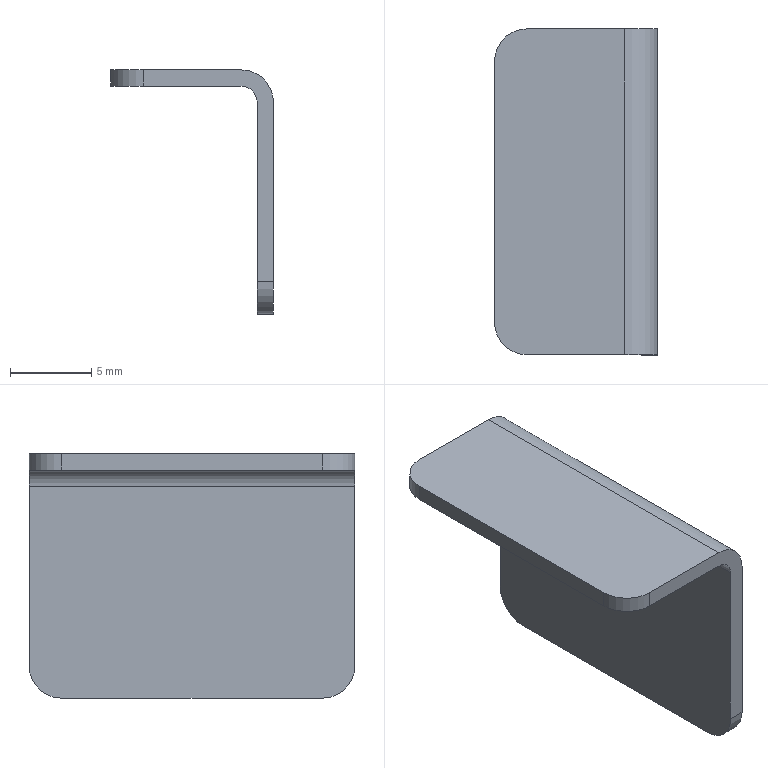Part | STEP file | Tube feed_id198_x_t | 1 solid | 14 faces | box 10 x 20 x 15 mm | volume 463.69 mm3 | plane 8 | cylinder 6 | commonest cylinder face diameters 4 x5 2 x1
STEP:
#1=CARTESIAN_POINT('',(0.,0.,0.));
#2=DIRECTION('',(0.,0.,1.));
#3=DIRECTION('',(1.,0.,0.));
#4=AXIS2_PLACEMENT_3D('',#1,#2,#3);
#5=CARTESIAN_POINT('',(16.,419.936,-21.));
#6=VERTEX_POINT('',#5);
#7=CARTESIAN_POINT('',(16.,403.936,-21.));
#8=VERTEX_POINT('',#7);
#9=CARTESIAN_POINT('',(16.,415.936,-21.));
#10=DIRECTION('',(0.,-1.,0.));
#11=VECTOR('',#10,1.);
#12=LINE('',#9,#11);
#13=CARTESIAN_POINT('',(16.,415.936,-21.));
#14=DIRECTION('',(-1.,0.,0.));
#15=DIRECTION('',(0.,-1.,0.));
#16=AXIS2_PLACEMENT_3D('',#13,#14,#15);
#17=PLANE('',#16);
#18=CARTESIAN_POINT('',(0.,0.));
#19=DIRECTION('',(1.,0.));
#20=VECTOR('',#19,1.);
#21=LINE('',#18,#20);
#22=(GEOMETRIC_REPRESENTATION_CONTEXT(2)PARAMETRIC_REPRESENTATION_CONTEXT()REPRESENTATION_CONTEXT('',''));
#23=DEFINITIONAL_REPRESENTATION('',(#21),#22);
#24=PCURVE('',#17,#23);
#25=CARTESIAN_POINT('',(24.,415.936,-21.));
#26=DIRECTION('',(0.,0.,1.));
#27=DIRECTION('',(1.,0.,0.));
#28=AXIS2_PLACEMENT_3D('',#25,#26,#27);
#29=PLANE('',#28);
#30=CARTESIAN_POINT('',(-8.,0.));
#31=DIRECTION('',(0.,-1.));
#32=VECTOR('',#31,1.);
#33=LINE('',#30,#32);
#34=(GEOMETRIC_REPRESENTATION_CONTEXT(2)PARAMETRIC_REPRESENTATION_CONTEXT()REPRESENTATION_CONTEXT('',''));
#35=DEFINITIONAL_REPRESENTATION('',(#33),#34);
#36=PCURVE('',#29,#35);
#37=SURFACE_CURVE('',#12,(#24,#36),.PCURVE_S1.);
#38=EDGE_CURVE('',#6,#8,#37,.T.);
#39=ORIENTED_EDGE('',*,*,#38,.F.);
#40=CARTESIAN_POINT('',(16.,419.936,-22.));
#41=VERTEX_POINT('',#40);
#42=CARTESIAN_POINT('',(16.,419.936,-21.));
#43=DIRECTION('',(0.,0.,-1.));
#44=VECTOR('',#43,1.);
#45=LINE('',#42,#44);
#46=CARTESIAN_POINT('',(-4.,0.));
#47=DIRECTION('',(0.,-1.));
#48=VECTOR('',#47,1.);
#49=LINE('',#46,#48);
#50=(GEOMETRIC_REPRESENTATION_CONTEXT(2)PARAMETRIC_REPRESENTATION_CONTEXT()REPRESENTATION_CONTEXT('',''));
#51=DEFINITIONAL_REPRESENTATION('',(#49),#50);
#52=PCURVE('',#17,#51);
#53=CARTESIAN_POINT('',(18.,419.936,-21.));
#54=DIRECTION('',(0.,0.,-1.));
#55=DIRECTION('',(-1.,0.,0.));
#56=AXIS2_PLACEMENT_3D('',#53,#54,#55);
#57=CYLINDRICAL_SURFACE('',#56,2.);
#58=CARTESIAN_POINT('',(0.,0.));
#59=DIRECTION('',(0.,1.));
#60=VECTOR('',#59,1.);
#61=LINE('',#58,#60);
#62=(GEOMETRIC_REPRESENTATION_CONTEXT(2)PARAMETRIC_REPRESENTATION_CONTEXT()REPRESENTATION_CONTEXT('',''));
#63=DEFINITIONAL_REPRESENTATION('',(#61),#62);
#64=PCURVE('',#57,#63);
#65=SURFACE_CURVE('',#45,(#52,#64),.PCURVE_S1.);
#66=EDGE_CURVE('',#6,#41,#65,.T.);
#67=ORIENTED_EDGE('',*,*,#66,.T.);
#68=CARTESIAN_POINT('',(16.,403.936,-22.));
#69=VERTEX_POINT('',#68);
#70=CARTESIAN_POINT('',(16.,415.936,-22.));
#71=DIRECTION('',(0.,-1.,0.));
#72=VECTOR('',#71,1.);
#73=LINE('',#70,#72);
#74=CARTESIAN_POINT('',(0.,-1.));
#75=DIRECTION('',(1.,0.));
#76=VECTOR('',#75,1.);
#77=LINE('',#74,#76);
#78=(GEOMETRIC_REPRESENTATION_CONTEXT(2)PARAMETRIC_REPRESENTATION_CONTEXT()REPRESENTATION_CONTEXT('',''));
#79=DEFINITIONAL_REPRESENTATION('',(#77),#78);
#80=PCURVE('',#17,#79);
#81=CARTESIAN_POINT('',(24.,415.936,-22.));
#82=DIRECTION('',(0.,0.,1.));
#83=DIRECTION('',(1.,0.,0.));
#84=AXIS2_PLACEMENT_3D('',#81,#82,#83);
#85=PLANE('',#84);
#86=CARTESIAN_POINT('',(-8.,0.));
#87=DIRECTION('',(0.,-1.));
#88=VECTOR('',#87,1.);
#89=LINE('',#86,#88);
#90=(GEOMETRIC_REPRESENTATION_CONTEXT(2)PARAMETRIC_REPRESENTATION_CONTEXT()REPRESENTATION_CONTEXT('',''));
#91=DEFINITIONAL_REPRESENTATION('',(#89),#90);
#92=PCURVE('',#85,#91);
#93=SURFACE_CURVE('',#73,(#80,#92),.PCURVE_S1.);
#94=EDGE_CURVE('',#41,#69,#93,.T.);
#95=ORIENTED_EDGE('',*,*,#94,.T.);
#96=CARTESIAN_POINT('',(16.,403.936,-21.));
#97=DIRECTION('',(0.,0.,1.));
#98=VECTOR('',#97,1.);
#99=LINE('',#96,#98);
#100=CARTESIAN_POINT('',(12.,0.));
#101=DIRECTION('',(0.,1.));
#102=VECTOR('',#101,1.);
#103=LINE('',#100,#102);
#104=(GEOMETRIC_REPRESENTATION_CONTEXT(2)PARAMETRIC_REPRESENTATION_CONTEXT()REPRESENTATION_CONTEXT('',''));
#105=DEFINITIONAL_REPRESENTATION('',(#103),#104);
#106=PCURVE('',#17,#105);
#107=CARTESIAN_POINT('',(18.,403.936,-23.));
#108=DIRECTION('',(0.,0.,1.));
#109=DIRECTION('',(0.,-1.,0.));
#110=AXIS2_PLACEMENT_3D('',#107,#108,#109);
#111=CYLINDRICAL_SURFACE('',#110,2.);
#112=CARTESIAN_POINT('',(4.712,2.));
#113=DIRECTION('',(0.,1.));
#114=VECTOR('',#113,1.);
#115=LINE('',#112,#114);
#116=(GEOMETRIC_REPRESENTATION_CONTEXT(2)PARAMETRIC_REPRESENTATION_CONTEXT()REPRESENTATION_CONTEXT('',''));
#117=DEFINITIONAL_REPRESENTATION('',(#115),#116);
#118=PCURVE('',#111,#117);
#119=SURFACE_CURVE('',#99,(#106,#118),.PCURVE_S1.);
#120=EDGE_CURVE('',#69,#8,#119,.T.);
#121=ORIENTED_EDGE('',*,*,#120,.T.);
#122=EDGE_LOOP('',(#39,#67,#95,#121));
#123=FACE_BOUND('',#122,.T.);
#124=ADVANCED_FACE('',(#123),#17,.T.);
#125=CARTESIAN_POINT('',(24.,421.936,-22.));
#126=VERTEX_POINT('',#125);
#127=CARTESIAN_POINT('',(18.,421.936,-22.));
#128=VERTEX_POINT('',#127);
#129=CARTESIAN_POINT('',(24.,421.936,-22.));
#130=DIRECTION('',(-1.,0.,0.));
#131=VECTOR('',#130,1.);
#132=LINE('',#129,#131);
#133=CARTESIAN_POINT('',(0.,421.936,0.));
#134=DIRECTION('',(0.,1.,0.));
#135=DIRECTION('',(0.,0.,1.));
#136=AXIS2_PLACEMENT_3D('',#133,#134,#135);
#137=PLANE('',#136);
#138=CARTESIAN_POINT('',(-22.,24.));
#139=DIRECTION('',(0.,-1.));
#140=VECTOR('',#139,1.);
#141=LINE('',#138,#140);
#142=(GEOMETRIC_REPRESENTATION_CONTEXT(2)PARAMETRIC_REPRESENTATION_CONTEXT()REPRESENTATION_CONTEXT('',''));
#143=DEFINITIONAL_REPRESENTATION('',(#141),#142);
#144=PCURVE('',#137,#143);
#145=CARTESIAN_POINT('',(0.,6.));
#146=DIRECTION('',(-1.,0.));
#147=VECTOR('',#146,1.);
#148=LINE('',#145,#147);
#149=(GEOMETRIC_REPRESENTATION_CONTEXT(2)PARAMETRIC_REPRESENTATION_CONTEXT()REPRESENTATION_CONTEXT('',''));
#150=DEFINITIONAL_REPRESENTATION('',(#148),#149);
#151=PCURVE('',#85,#150);
#152=SURFACE_CURVE('',#132,(#144,#151),.PCURVE_S1.);
#153=EDGE_CURVE('',#126,#128,#152,.T.);
#154=ORIENTED_EDGE('',*,*,#153,.T.);
#155=CARTESIAN_POINT('',(18.,421.936,-21.));
#156=VERTEX_POINT('',#155);
#157=CARTESIAN_POINT('',(18.,421.936,0.));
#158=DIRECTION('',(0.,0.,1.));
#159=VECTOR('',#158,1.);
#160=LINE('',#157,#159);
#161=CARTESIAN_POINT('',(0.,18.));
#162=DIRECTION('',(1.,0.));
#163=VECTOR('',#162,1.);
#164=LINE('',#161,#163);
#165=(GEOMETRIC_REPRESENTATION_CONTEXT(2)PARAMETRIC_REPRESENTATION_CONTEXT()REPRESENTATION_CONTEXT('',''));
#166=DEFINITIONAL_REPRESENTATION('',(#164),#165);
#167=PCURVE('',#137,#166);
#168=CARTESIAN_POINT('',(1.571,-21.));
#169=DIRECTION('',(0.,-1.));
#170=VECTOR('',#169,1.);
#171=LINE('',#168,#170);
#172=(GEOMETRIC_REPRESENTATION_CONTEXT(2)PARAMETRIC_REPRESENTATION_CONTEXT()REPRESENTATION_CONTEXT('',''));
#173=DEFINITIONAL_REPRESENTATION('',(#171),#172);
#174=PCURVE('',#57,#173);
#175=SURFACE_CURVE('',#160,(#167,#174),.PCURVE_S1.);
#176=EDGE_CURVE('',#128,#156,#175,.T.);
#177=ORIENTED_EDGE('',*,*,#176,.T.);
#178=CARTESIAN_POINT('',(24.,421.936,-21.));
#179=VERTEX_POINT('',#178);
#180=CARTESIAN_POINT('',(24.,421.936,-21.));
#181=DIRECTION('',(-1.,0.,0.));
#182=VECTOR('',#181,1.);
#183=LINE('',#180,#182);
#184=CARTESIAN_POINT('',(-21.,24.));
#185=DIRECTION('',(0.,-1.));
#186=VECTOR('',#185,1.);
#187=LINE('',#184,#186);
#188=(GEOMETRIC_REPRESENTATION_CONTEXT(2)PARAMETRIC_REPRESENTATION_CONTEXT()REPRESENTATION_CONTEXT('',''));
#189=DEFINITIONAL_REPRESENTATION('',(#187),#188);
#190=PCURVE('',#137,#189);
#191=CARTESIAN_POINT('',(0.,6.));
#192=DIRECTION('',(-1.,0.));
#193=VECTOR('',#192,1.);
#194=LINE('',#191,#193);
#195=(GEOMETRIC_REPRESENTATION_CONTEXT(2)PARAMETRIC_REPRESENTATION_CONTEXT()REPRESENTATION_CONTEXT('',''));
#196=DEFINITIONAL_REPRESENTATION('',(#194),#195);
#197=PCURVE('',#29,#196);
#198=SURFACE_CURVE('',#183,(#190,#197),.PCURVE_S1.);
#199=EDGE_CURVE('',#179,#156,#198,.T.);
#200=ORIENTED_EDGE('',*,*,#199,.F.);
#201=CARTESIAN_POINT('',(26.,421.936,-23.));
#202=VERTEX_POINT('',#201);
#203=CARTESIAN_POINT('',(24.,421.936,-23.));
#204=DIRECTION('',(0.,-1.,0.));
#205=DIRECTION('',(0.,0.,1.));
#206=AXIS2_PLACEMENT_3D('',#203,#204,#205);
#207=CIRCLE('',#206,2.);
#208=CARTESIAN_POINT('',(-21.,24.));
#209=CARTESIAN_POINT('',(-21.,20.536));
#210=CARTESIAN_POINT('',(-24.,22.268));
#211=CARTESIAN_POINT('',(-27.,24.));
#212=CARTESIAN_POINT('',(-24.,25.732));
#213=CARTESIAN_POINT('',(-21.,27.464));
#214=CARTESIAN_POINT('',(-21.,24.));
#215=(BOUNDED_CURVE()B_SPLINE_CURVE(2,(#208,#209,#210,#211,#212,#213,#214),.UNSPECIFIED.,.T.,.F.)B_SPLINE_CURVE_WITH_KNOTS((1,2,2,2,2,1),(-2.094,0.,2.094,4.189,6.283,8.378),.UNSPECIFIED.)CURVE()GEOMETRIC_REPRESENTATION_ITEM()RATIONAL_B_SPLINE_CURVE((1.,0.5,1.,0.5,1.,0.5,1.))REPRESENTATION_ITEM(''));
#216=(GEOMETRIC_REPRESENTATION_CONTEXT(2)PARAMETRIC_REPRESENTATION_CONTEXT()REPRESENTATION_CONTEXT('',''));
#217=DEFINITIONAL_REPRESENTATION('',(#215),#216);
#218=PCURVE('',#137,#217);
#219=CARTESIAN_POINT('',(24.,415.936,-23.));
#220=DIRECTION('',(0.,-1.,0.));
#221=DIRECTION('',(0.,0.,-1.));
#222=AXIS2_PLACEMENT_3D('',#219,#220,#221);
#223=CYLINDRICAL_SURFACE('',#222,2.);
#224=CARTESIAN_POINT('',(-3.142,-6.));
#225=DIRECTION('',(1.,0.));
#226=VECTOR('',#225,1.);
#227=LINE('',#224,#226);
#228=(GEOMETRIC_REPRESENTATION_CONTEXT(2)PARAMETRIC_REPRESENTATION_CONTEXT()REPRESENTATION_CONTEXT('',''));
#229=DEFINITIONAL_REPRESENTATION('',(#227),#228);
#230=PCURVE('',#223,#229);
#231=SURFACE_CURVE('',#207,(#218,#230),.PCURVE_S1.);
#232=EDGE_CURVE('',#202,#179,#231,.T.);
#233=ORIENTED_EDGE('',*,*,#232,.F.);
#234=CARTESIAN_POINT('',(26.,421.936,-34.));
#235=VERTEX_POINT('',#234);
#236=CARTESIAN_POINT('',(26.,421.936,-36.));
#237=DIRECTION('',(0.,0.,1.));
#238=VECTOR('',#237,1.);
#239=LINE('',#236,#238);
#240=CARTESIAN_POINT('',(-36.,26.));
#241=DIRECTION('',(1.,0.));
#242=VECTOR('',#241,1.);
#243=LINE('',#240,#242);
#244=(GEOMETRIC_REPRESENTATION_CONTEXT(2)PARAMETRIC_REPRESENTATION_CONTEXT()REPRESENTATION_CONTEXT('',''));
#245=DEFINITIONAL_REPRESENTATION('',(#243),#244);
#246=PCURVE('',#137,#245);
#247=CARTESIAN_POINT('',(26.,415.936,-36.));
#248=DIRECTION('',(1.,0.,0.));
#249=DIRECTION('',(0.,0.,-1.));
#250=AXIS2_PLACEMENT_3D('',#247,#248,#249);
#251=PLANE('',#250);
#252=CARTESIAN_POINT('',(0.,6.));
#253=DIRECTION('',(-1.,0.));
#254=VECTOR('',#253,1.);
#255=LINE('',#252,#254);
#256=(GEOMETRIC_REPRESENTATION_CONTEXT(2)PARAMETRIC_REPRESENTATION_CONTEXT()REPRESENTATION_CONTEXT('',''));
#257=DEFINITIONAL_REPRESENTATION('',(#255),#256);
#258=PCURVE('',#251,#257);
#259=SURFACE_CURVE('',#239,(#246,#258),.PCURVE_S1.);
#260=EDGE_CURVE('',#235,#202,#259,.T.);
#261=ORIENTED_EDGE('',*,*,#260,.F.);
#262=CARTESIAN_POINT('',(25.,421.936,-34.));
#263=VERTEX_POINT('',#262);
#264=CARTESIAN_POINT('',(0.,421.936,-34.));
#265=DIRECTION('',(-1.,0.,0.));
#266=VECTOR('',#265,1.);
#267=LINE('',#264,#266);
#268=CARTESIAN_POINT('',(-34.,0.));
#269=DIRECTION('',(0.,-1.));
#270=VECTOR('',#269,1.);
#271=LINE('',#268,#270);
#272=(GEOMETRIC_REPRESENTATION_CONTEXT(2)PARAMETRIC_REPRESENTATION_CONTEXT()REPRESENTATION_CONTEXT('',''));
#273=DEFINITIONAL_REPRESENTATION('',(#271),#272);
#274=PCURVE('',#137,#273);
#275=CARTESIAN_POINT('',(0.,419.936,-34.));
#276=DIRECTION('',(1.,0.,0.));
#277=DIRECTION('',(0.,0.,-1.));
#278=AXIS2_PLACEMENT_3D('',#275,#276,#277);
#279=CYLINDRICAL_SURFACE('',#278,2.);
#280=CARTESIAN_POINT('',(1.571,0.));
#281=DIRECTION('',(0.,-1.));
#282=VECTOR('',#281,1.);
#283=LINE('',#280,#282);
#284=(GEOMETRIC_REPRESENTATION_CONTEXT(2)PARAMETRIC_REPRESENTATION_CONTEXT()REPRESENTATION_CONTEXT('',''));
#285=DEFINITIONAL_REPRESENTATION('',(#283),#284);
#286=PCURVE('',#279,#285);
#287=SURFACE_CURVE('',#267,(#274,#286),.PCURVE_S1.);
#288=EDGE_CURVE('',#235,#263,#287,.T.);
#289=ORIENTED_EDGE('',*,*,#288,.T.);
#290=CARTESIAN_POINT('',(25.,421.936,-23.));
#291=VERTEX_POINT('',#290);
#292=CARTESIAN_POINT('',(25.,421.936,-36.));
#293=DIRECTION('',(0.,0.,1.));
#294=VECTOR('',#293,1.);
#295=LINE('',#292,#294);
#296=CARTESIAN_POINT('',(-36.,25.));
#297=DIRECTION('',(1.,0.));
#298=VECTOR('',#297,1.);
#299=LINE('',#296,#298);
#300=(GEOMETRIC_REPRESENTATION_CONTEXT(2)PARAMETRIC_REPRESENTATION_CONTEXT()REPRESENTATION_CONTEXT('',''));
#301=DEFINITIONAL_REPRESENTATION('',(#299),#300);
#302=PCURVE('',#137,#301);
#303=CARTESIAN_POINT('',(25.,415.936,-36.));
#304=DIRECTION('',(1.,0.,0.));
#305=DIRECTION('',(0.,0.,-1.));
#306=AXIS2_PLACEMENT_3D('',#303,#304,#305);
#307=PLANE('',#306);
#308=CARTESIAN_POINT('',(0.,6.));
#309=DIRECTION('',(-1.,0.));
#310=VECTOR('',#309,1.);
#311=LINE('',#308,#310);
#312=(GEOMETRIC_REPRESENTATION_CONTEXT(2)PARAMETRIC_REPRESENTATION_CONTEXT()REPRESENTATION_CONTEXT('',''));
#313=DEFINITIONAL_REPRESENTATION('',(#311),#312);
#314=PCURVE('',#307,#313);
#315=SURFACE_CURVE('',#295,(#302,#314),.PCURVE_S1.);
#316=EDGE_CURVE('',#263,#291,#315,.T.);
#317=ORIENTED_EDGE('',*,*,#316,.T.);
#318=CARTESIAN_POINT('',(24.,421.936,-23.));
#319=DIRECTION('',(0.,-1.,0.));
#320=DIRECTION('',(0.,0.,1.));
#321=AXIS2_PLACEMENT_3D('',#318,#319,#320);
#322=CIRCLE('',#321,1.);
#323=CARTESIAN_POINT('',(-22.,24.));
#324=CARTESIAN_POINT('',(-22.,22.268));
#325=CARTESIAN_POINT('',(-23.5,23.134));
#326=CARTESIAN_POINT('',(-25.,24.));
#327=CARTESIAN_POINT('',(-23.5,24.866));
#328=CARTESIAN_POINT('',(-22.,25.732));
#329=CARTESIAN_POINT('',(-22.,24.));
#330=(BOUNDED_CURVE()B_SPLINE_CURVE(2,(#323,#324,#325,#326,#327,#328,#329),.UNSPECIFIED.,.T.,.F.)B_SPLINE_CURVE_WITH_KNOTS((1,2,2,2,2,1),(-2.094,0.,2.094,4.189,6.283,8.378),.UNSPECIFIED.)CURVE()GEOMETRIC_REPRESENTATION_ITEM()RATIONAL_B_SPLINE_CURVE((1.,0.5,1.,0.5,1.,0.5,1.))REPRESENTATION_ITEM(''));
#331=(GEOMETRIC_REPRESENTATION_CONTEXT(2)PARAMETRIC_REPRESENTATION_CONTEXT()REPRESENTATION_CONTEXT('',''));
#332=DEFINITIONAL_REPRESENTATION('',(#330),#331);
#333=PCURVE('',#137,#332);
#334=CARTESIAN_POINT('',(24.,415.936,-23.));
#335=DIRECTION('',(0.,-1.,0.));
#336=DIRECTION('',(0.,0.,-1.));
#337=AXIS2_PLACEMENT_3D('',#334,#335,#336);
#338=CYLINDRICAL_SURFACE('',#337,1.);
#339=CARTESIAN_POINT('',(-3.142,-6.));
#340=DIRECTION('',(1.,0.));
#341=VECTOR('',#340,1.);
#342=LINE('',#339,#341);
#343=(GEOMETRIC_REPRESENTATION_CONTEXT(2)PARAMETRIC_REPRESENTATION_CONTEXT()REPRESENTATION_CONTEXT('',''));
#344=DEFINITIONAL_REPRESENTATION('',(#342),#343);
#345=PCURVE('',#338,#344);
#346=SURFACE_CURVE('',#322,(#333,#345),.PCURVE_S1.);
#347=EDGE_CURVE('',#291,#126,#346,.T.);
#348=ORIENTED_EDGE('',*,*,#347,.T.);
#349=EDGE_LOOP('',(#154,#177,#200,#233,#261,#289,#317,#348));
#350=FACE_BOUND('',#349,.T.);
#351=ADVANCED_FACE('',(#350),#137,.T.);
#352=CARTESIAN_POINT('',(26.,419.936,-36.));
#353=VERTEX_POINT('',#352);
#354=CARTESIAN_POINT('',(26.,403.936,-36.));
#355=VERTEX_POINT('',#354);
#356=CARTESIAN_POINT('',(26.,415.936,-36.));
#357=DIRECTION('',(0.,-1.,0.));
#358=VECTOR('',#357,1.);
#359=LINE('',#356,#358);
#360=CARTESIAN_POINT('',(26.,415.936,-36.));
#361=DIRECTION('',(0.,0.,1.));
#362=DIRECTION('',(0.,-1.,0.));
#363=AXIS2_PLACEMENT_3D('',#360,#361,#362);
#364=PLANE('',#363);
#365=CARTESIAN_POINT('',(0.,0.));
#366=DIRECTION('',(1.,0.));
#367=VECTOR('',#366,1.);
#368=LINE('',#365,#367);
#369=(GEOMETRIC_REPRESENTATION_CONTEXT(2)PARAMETRIC_REPRESENTATION_CONTEXT()REPRESENTATION_CONTEXT('',''));
#370=DEFINITIONAL_REPRESENTATION('',(#368),#369);
#371=PCURVE('',#364,#370);
#372=CARTESIAN_POINT('',(0.,0.));
#373=DIRECTION('',(0.,-1.));
#374=VECTOR('',#373,1.);
#375=LINE('',#372,#374);
#376=(GEOMETRIC_REPRESENTATION_CONTEXT(2)PARAMETRIC_REPRESENTATION_CONTEXT()REPRESENTATION_CONTEXT('',''));
#377=DEFINITIONAL_REPRESENTATION('',(#375),#376);
#378=PCURVE('',#251,#377);
#379=SURFACE_CURVE('',#359,(#371,#378),.PCURVE_S1.);
#380=EDGE_CURVE('',#353,#355,#379,.T.);
#381=ORIENTED_EDGE('',*,*,#380,.T.);
#382=CARTESIAN_POINT('',(25.,403.936,-36.));
#383=VERTEX_POINT('',#382);
#384=CARTESIAN_POINT('',(26.,403.936,-36.));
#385=DIRECTION('',(-1.,0.,0.));
#386=VECTOR('',#385,1.);
#387=LINE('',#384,#386);
#388=CARTESIAN_POINT('',(12.,0.));
#389=DIRECTION('',(0.,-1.));
#390=VECTOR('',#389,1.);
#391=LINE('',#388,#390);
#392=(GEOMETRIC_REPRESENTATION_CONTEXT(2)PARAMETRIC_REPRESENTATION_CONTEXT()REPRESENTATION_CONTEXT('',''));
#393=DEFINITIONAL_REPRESENTATION('',(#391),#392);
#394=PCURVE('',#364,#393);
#395=CARTESIAN_POINT('',(26.,403.936,-34.));
#396=DIRECTION('',(-1.,0.,0.));
#397=DIRECTION('',(0.,0.,1.));
#398=AXIS2_PLACEMENT_3D('',#395,#396,#397);
#399=CYLINDRICAL_SURFACE('',#398,2.);
#400=CARTESIAN_POINT('',(3.142,0.));
#401=DIRECTION('',(0.,1.));
#402=VECTOR('',#401,1.);
#403=LINE('',#400,#402);
#404=(GEOMETRIC_REPRESENTATION_CONTEXT(2)PARAMETRIC_REPRESENTATION_CONTEXT()REPRESENTATION_CONTEXT('',''));
#405=DEFINITIONAL_REPRESENTATION('',(#403),#404);
#406=PCURVE('',#399,#405);
#407=SURFACE_CURVE('',#387,(#394,#406),.PCURVE_S1.);
#408=EDGE_CURVE('',#355,#383,#407,.T.);
#409=ORIENTED_EDGE('',*,*,#408,.T.);
#410=CARTESIAN_POINT('',(25.,419.936,-36.));
#411=VERTEX_POINT('',#410);
#412=CARTESIAN_POINT('',(25.,415.936,-36.));
#413=DIRECTION('',(0.,-1.,0.));
#414=VECTOR('',#413,1.);
#415=LINE('',#412,#414);
#416=CARTESIAN_POINT('',(0.,-1.));
#417=DIRECTION('',(1.,0.));
#418=VECTOR('',#417,1.);
#419=LINE('',#416,#418);
#420=(GEOMETRIC_REPRESENTATION_CONTEXT(2)PARAMETRIC_REPRESENTATION_CONTEXT()REPRESENTATION_CONTEXT('',''));
#421=DEFINITIONAL_REPRESENTATION('',(#419),#420);
#422=PCURVE('',#364,#421);
#423=CARTESIAN_POINT('',(0.,0.));
#424=DIRECTION('',(0.,-1.));
#425=VECTOR('',#424,1.);
#426=LINE('',#423,#425);
#427=(GEOMETRIC_REPRESENTATION_CONTEXT(2)PARAMETRIC_REPRESENTATION_CONTEXT()REPRESENTATION_CONTEXT('',''));
#428=DEFINITIONAL_REPRESENTATION('',(#426),#427);
#429=PCURVE('',#307,#428);
#430=SURFACE_CURVE('',#415,(#422,#429),.PCURVE_S1.);
#431=EDGE_CURVE('',#411,#383,#430,.T.);
#432=ORIENTED_EDGE('',*,*,#431,.F.);
#433=CARTESIAN_POINT('',(26.,419.936,-36.));
#434=DIRECTION('',(1.,0.,0.));
#435=VECTOR('',#434,1.);
#436=LINE('',#433,#435);
#437=CARTESIAN_POINT('',(-4.,0.));
#438=DIRECTION('',(0.,1.));
#439=VECTOR('',#438,1.);
#440=LINE('',#437,#439);
#441=(GEOMETRIC_REPRESENTATION_CONTEXT(2)PARAMETRIC_REPRESENTATION_CONTEXT()REPRESENTATION_CONTEXT('',''));
#442=DEFINITIONAL_REPRESENTATION('',(#440),#441);
#443=PCURVE('',#364,#442);
#444=CARTESIAN_POINT('',(0.,26.));
#445=DIRECTION('',(0.,1.));
#446=VECTOR('',#445,1.);
#447=LINE('',#444,#446);
#448=(GEOMETRIC_REPRESENTATION_CONTEXT(2)PARAMETRIC_REPRESENTATION_CONTEXT()REPRESENTATION_CONTEXT('',''));
#449=DEFINITIONAL_REPRESENTATION('',(#447),#448);
#450=PCURVE('',#279,#449);
#451=SURFACE_CURVE('',#436,(#443,#450),.PCURVE_S1.);
#452=EDGE_CURVE('',#411,#353,#451,.T.);
#453=ORIENTED_EDGE('',*,*,#452,.T.);
#454=EDGE_LOOP('',(#381,#409,#432,#453));
#455=FACE_BOUND('',#454,.T.);
#456=ADVANCED_FACE('',(#455),#364,.F.);
#457=CARTESIAN_POINT('',(24.,401.936,-21.));
#458=VERTEX_POINT('',#457);
#459=CARTESIAN_POINT('',(18.,401.936,-21.));
#460=VERTEX_POINT('',#459);
#461=CARTESIAN_POINT('',(24.,401.936,-21.));
#462=DIRECTION('',(-1.,0.,0.));
#463=VECTOR('',#462,1.);
#464=LINE('',#461,#463);
#465=CARTESIAN_POINT('',(24.,401.936,-23.));
#466=DIRECTION('',(0.,1.,0.));
#467=DIRECTION('',(0.,0.,1.));
#468=AXIS2_PLACEMENT_3D('',#465,#466,#467);
#469=PLANE('',#468);
#470=CARTESIAN_POINT('',(2.,0.));
#471=DIRECTION('',(0.,-1.));
#472=VECTOR('',#471,1.);
#473=LINE('',#470,#472);
#474=(GEOMETRIC_REPRESENTATION_CONTEXT(2)PARAMETRIC_REPRESENTATION_CONTEXT()REPRESENTATION_CONTEXT('',''));
#475=DEFINITIONAL_REPRESENTATION('',(#473),#474);
#476=PCURVE('',#469,#475);
#477=CARTESIAN_POINT('',(0.,-14.));
#478=DIRECTION('',(-1.,0.));
#479=VECTOR('',#478,1.);
#480=LINE('',#477,#479);
#481=(GEOMETRIC_REPRESENTATION_CONTEXT(2)PARAMETRIC_REPRESENTATION_CONTEXT()REPRESENTATION_CONTEXT('',''));
#482=DEFINITIONAL_REPRESENTATION('',(#480),#481);
#483=PCURVE('',#29,#482);
#484=SURFACE_CURVE('',#464,(#476,#483),.PCURVE_S1.);
#485=EDGE_CURVE('',#458,#460,#484,.T.);
#486=ORIENTED_EDGE('',*,*,#485,.T.);
#487=CARTESIAN_POINT('',(18.,401.936,-22.));
#488=VERTEX_POINT('',#487);
#489=CARTESIAN_POINT('',(18.,401.936,-23.));
#490=DIRECTION('',(0.,0.,-1.));
#491=VECTOR('',#490,1.);
#492=LINE('',#489,#491);
#493=CARTESIAN_POINT('',(0.,-6.));
#494=DIRECTION('',(-1.,0.));
#495=VECTOR('',#494,1.);
#496=LINE('',#493,#495);
#497=(GEOMETRIC_REPRESENTATION_CONTEXT(2)PARAMETRIC_REPRESENTATION_CONTEXT()REPRESENTATION_CONTEXT('',''));
#498=DEFINITIONAL_REPRESENTATION('',(#496),#497);
#499=PCURVE('',#469,#498);
#500=CARTESIAN_POINT('',(6.283,0.));
#501=DIRECTION('',(0.,-1.));
#502=VECTOR('',#501,1.);
#503=LINE('',#500,#502);
#504=(GEOMETRIC_REPRESENTATION_CONTEXT(2)PARAMETRIC_REPRESENTATION_CONTEXT()REPRESENTATION_CONTEXT('',''));
#505=DEFINITIONAL_REPRESENTATION('',(#503),#504);
#506=PCURVE('',#111,#505);
#507=SURFACE_CURVE('',#492,(#499,#506),.PCURVE_S1.);
#508=EDGE_CURVE('',#460,#488,#507,.T.);
#509=ORIENTED_EDGE('',*,*,#508,.T.);
#510=CARTESIAN_POINT('',(24.,401.936,-22.));
#511=VERTEX_POINT('',#510);
#512=CARTESIAN_POINT('',(24.,401.936,-22.));
#513=DIRECTION('',(-1.,0.,0.));
#514=VECTOR('',#513,1.);
#515=LINE('',#512,#514);
#516=CARTESIAN_POINT('',(1.,0.));
#517=DIRECTION('',(0.,-1.));
#518=VECTOR('',#517,1.);
#519=LINE('',#516,#518);
#520=(GEOMETRIC_REPRESENTATION_CONTEXT(2)PARAMETRIC_REPRESENTATION_CONTEXT()REPRESENTATION_CONTEXT('',''));
#521=DEFINITIONAL_REPRESENTATION('',(#519),#520);
#522=PCURVE('',#469,#521);
#523=CARTESIAN_POINT('',(0.,-14.));
#524=DIRECTION('',(-1.,0.));
#525=VECTOR('',#524,1.);
#526=LINE('',#523,#525);
#527=(GEOMETRIC_REPRESENTATION_CONTEXT(2)PARAMETRIC_REPRESENTATION_CONTEXT()REPRESENTATION_CONTEXT('',''));
#528=DEFINITIONAL_REPRESENTATION('',(#526),#527);
#529=PCURVE('',#85,#528);
#530=SURFACE_CURVE('',#515,(#522,#529),.PCURVE_S1.);
#531=EDGE_CURVE('',#511,#488,#530,.T.);
#532=ORIENTED_EDGE('',*,*,#531,.F.);
#533=CARTESIAN_POINT('',(25.,401.936,-23.));
#534=VERTEX_POINT('',#533);
#535=CARTESIAN_POINT('',(24.,401.936,-23.));
#536=DIRECTION('',(0.,-1.,0.));
#537=DIRECTION('',(0.,0.,1.));
#538=AXIS2_PLACEMENT_3D('',#535,#536,#537);
#539=CIRCLE('',#538,1.);
#540=CARTESIAN_POINT('',(1.,0.));
#541=CARTESIAN_POINT('',(1.,-1.732));
#542=CARTESIAN_POINT('',(-0.5,-0.866));
#543=CARTESIAN_POINT('',(-2.,0.));
#544=CARTESIAN_POINT('',(-0.5,0.866));
#545=CARTESIAN_POINT('',(1.,1.732));
#546=CARTESIAN_POINT('',(1.,0.));
#547=(BOUNDED_CURVE()B_SPLINE_CURVE(2,(#540,#541,#542,#543,#544,#545,#546),.UNSPECIFIED.,.T.,.F.)B_SPLINE_CURVE_WITH_KNOTS((1,2,2,2,2,1),(-2.094,0.,2.094,4.189,6.283,8.378),.UNSPECIFIED.)CURVE()GEOMETRIC_REPRESENTATION_ITEM()RATIONAL_B_SPLINE_CURVE((1.,0.5,1.,0.5,1.,0.5,1.))REPRESENTATION_ITEM(''));
#548=(GEOMETRIC_REPRESENTATION_CONTEXT(2)PARAMETRIC_REPRESENTATION_CONTEXT()REPRESENTATION_CONTEXT('',''));
#549=DEFINITIONAL_REPRESENTATION('',(#547),#548);
#550=PCURVE('',#469,#549);
#551=CARTESIAN_POINT('',(-3.142,14.));
#552=DIRECTION('',(1.,0.));
#553=VECTOR('',#552,1.);
#554=LINE('',#551,#553);
#555=(GEOMETRIC_REPRESENTATION_CONTEXT(2)PARAMETRIC_REPRESENTATION_CONTEXT()REPRESENTATION_CONTEXT('',''));
#556=DEFINITIONAL_REPRESENTATION('',(#554),#555);
#557=PCURVE('',#338,#556);
#558=SURFACE_CURVE('',#539,(#550,#557),.PCURVE_S1.);
#559=EDGE_CURVE('',#534,#511,#558,.T.);
#560=ORIENTED_EDGE('',*,*,#559,.F.);
#561=CARTESIAN_POINT('',(25.,401.936,-34.));
#562=VERTEX_POINT('',#561);
#563=CARTESIAN_POINT('',(25.,401.936,-23.));
#564=DIRECTION('',(0.,0.,1.));
#565=VECTOR('',#564,1.);
#566=LINE('',#563,#565);
#567=CARTESIAN_POINT('',(0.,1.));
#568=DIRECTION('',(1.,0.));
#569=VECTOR('',#568,1.);
#570=LINE('',#567,#569);
#571=(GEOMETRIC_REPRESENTATION_CONTEXT(2)PARAMETRIC_REPRESENTATION_CONTEXT()REPRESENTATION_CONTEXT('',''));
#572=DEFINITIONAL_REPRESENTATION('',(#570),#571);
#573=PCURVE('',#469,#572);
#574=CARTESIAN_POINT('',(-13.,-14.));
#575=DIRECTION('',(-1.,0.));
#576=VECTOR('',#575,1.);
#577=LINE('',#574,#576);
#578=(GEOMETRIC_REPRESENTATION_CONTEXT(2)PARAMETRIC_REPRESENTATION_CONTEXT()REPRESENTATION_CONTEXT('',''));
#579=DEFINITIONAL_REPRESENTATION('',(#577),#578);
#580=PCURVE('',#307,#579);
#581=SURFACE_CURVE('',#566,(#573,#580),.PCURVE_S1.);
#582=EDGE_CURVE('',#562,#534,#581,.T.);
#583=ORIENTED_EDGE('',*,*,#582,.F.);
#584=CARTESIAN_POINT('',(26.,401.936,-34.));
#585=VERTEX_POINT('',#584);
#586=CARTESIAN_POINT('',(24.,401.936,-34.));
#587=DIRECTION('',(1.,0.,0.));
#588=VECTOR('',#587,1.);
#589=LINE('',#586,#588);
#590=CARTESIAN_POINT('',(-11.,0.));
#591=DIRECTION('',(0.,1.));
#592=VECTOR('',#591,1.);
#593=LINE('',#590,#592);
#594=(GEOMETRIC_REPRESENTATION_CONTEXT(2)PARAMETRIC_REPRESENTATION_CONTEXT()REPRESENTATION_CONTEXT('',''));
#595=DEFINITIONAL_REPRESENTATION('',(#593),#594);
#596=PCURVE('',#469,#595);
#597=CARTESIAN_POINT('',(4.712,2.));
#598=DIRECTION('',(0.,-1.));
#599=VECTOR('',#598,1.);
#600=LINE('',#597,#599);
#601=(GEOMETRIC_REPRESENTATION_CONTEXT(2)PARAMETRIC_REPRESENTATION_CONTEXT()REPRESENTATION_CONTEXT('',''));
#602=DEFINITIONAL_REPRESENTATION('',(#600),#601);
#603=PCURVE('',#399,#602);
#604=SURFACE_CURVE('',#589,(#596,#603),.PCURVE_S1.);
#605=EDGE_CURVE('',#562,#585,#604,.T.);
#606=ORIENTED_EDGE('',*,*,#605,.T.);
#607=CARTESIAN_POINT('',(26.,401.936,-23.));
#608=VERTEX_POINT('',#607);
#609=CARTESIAN_POINT('',(26.,401.936,-23.));
#610=DIRECTION('',(0.,0.,1.));
#611=VECTOR('',#610,1.);
#612=LINE('',#609,#611);
#613=CARTESIAN_POINT('',(0.,2.));
#614=DIRECTION('',(1.,0.));
#615=VECTOR('',#614,1.);
#616=LINE('',#613,#615);
#617=(GEOMETRIC_REPRESENTATION_CONTEXT(2)PARAMETRIC_REPRESENTATION_CONTEXT()REPRESENTATION_CONTEXT('',''));
#618=DEFINITIONAL_REPRESENTATION('',(#616),#617);
#619=PCURVE('',#469,#618);
#620=CARTESIAN_POINT('',(-13.,-14.));
#621=DIRECTION('',(-1.,0.));
#622=VECTOR('',#621,1.);
#623=LINE('',#620,#622);
#624=(GEOMETRIC_REPRESENTATION_CONTEXT(2)PARAMETRIC_REPRESENTATION_CONTEXT()REPRESENTATION_CONTEXT('',''));
#625=DEFINITIONAL_REPRESENTATION('',(#623),#624);
#626=PCURVE('',#251,#625);
#627=SURFACE_CURVE('',#612,(#619,#626),.PCURVE_S1.);
#628=EDGE_CURVE('',#585,#608,#627,.T.);
#629=ORIENTED_EDGE('',*,*,#628,.T.);
#630=CARTESIAN_POINT('',(24.,401.936,-23.));
#631=DIRECTION('',(0.,-1.,0.));
#632=DIRECTION('',(0.,0.,1.));
#633=AXIS2_PLACEMENT_3D('',#630,#631,#632);
#634=CIRCLE('',#633,2.);
#635=CARTESIAN_POINT('',(2.,0.));
#636=CARTESIAN_POINT('',(2.,-3.464));
#637=CARTESIAN_POINT('',(-1.,-1.732));
#638=CARTESIAN_POINT('',(-4.,0.));
#639=CARTESIAN_POINT('',(-1.,1.732));
#640=CARTESIAN_POINT('',(2.,3.464));
#641=CARTESIAN_POINT('',(2.,0.));
#642=(BOUNDED_CURVE()B_SPLINE_CURVE(2,(#635,#636,#637,#638,#639,#640,#641),.UNSPECIFIED.,.T.,.F.)B_SPLINE_CURVE_WITH_KNOTS((1,2,2,2,2,1),(-2.094,0.,2.094,4.189,6.283,8.378),.UNSPECIFIED.)CURVE()GEOMETRIC_REPRESENTATION_ITEM()RATIONAL_B_SPLINE_CURVE((1.,0.5,1.,0.5,1.,0.5,1.))REPRESENTATION_ITEM(''));
#643=(GEOMETRIC_REPRESENTATION_CONTEXT(2)PARAMETRIC_REPRESENTATION_CONTEXT()REPRESENTATION_CONTEXT('',''));
#644=DEFINITIONAL_REPRESENTATION('',(#642),#643);
#645=PCURVE('',#469,#644);
#646=CARTESIAN_POINT('',(-3.142,14.));
#647=DIRECTION('',(1.,0.));
#648=VECTOR('',#647,1.);
#649=LINE('',#646,#648);
#650=(GEOMETRIC_REPRESENTATION_CONTEXT(2)PARAMETRIC_REPRESENTATION_CONTEXT()REPRESENTATION_CONTEXT('',''));
#651=DEFINITIONAL_REPRESENTATION('',(#649),#650);
#652=PCURVE('',#223,#651);
#653=SURFACE_CURVE('',#634,(#645,#652),.PCURVE_S1.);
#654=EDGE_CURVE('',#608,#458,#653,.T.);
#655=ORIENTED_EDGE('',*,*,#654,.T.);
#656=EDGE_LOOP('',(#486,#509,#532,#560,#583,#606,#629,#655));
#657=FACE_BOUND('',#656,.T.);
#658=ADVANCED_FACE('',(#657),#469,.F.);
#659=ORIENTED_EDGE('',*,*,#431,.T.);
#660=CARTESIAN_POINT('',(25.,403.936,-34.));
#661=DIRECTION('',(-1.,0.,0.));
#662=DIRECTION('',(0.,0.,-1.));
#663=AXIS2_PLACEMENT_3D('',#660,#661,#662);
#664=CIRCLE('',#663,2.);
#665=CARTESIAN_POINT('',(0.,-12.));
#666=CARTESIAN_POINT('',(0.,-15.464));
#667=CARTESIAN_POINT('',(-3.,-13.732));
#668=CARTESIAN_POINT('',(-6.,-12.));
#669=CARTESIAN_POINT('',(-3.,-10.268));
#670=CARTESIAN_POINT('',(0.,-8.536));
#671=CARTESIAN_POINT('',(0.,-12.));
#672=(BOUNDED_CURVE()B_SPLINE_CURVE(2,(#665,#666,#667,#668,#669,#670,#671),.UNSPECIFIED.,.T.,.F.)B_SPLINE_CURVE_WITH_KNOTS((1,2,2,2,2,1),(-2.094,0.,2.094,4.189,6.283,8.378),.UNSPECIFIED.)CURVE()GEOMETRIC_REPRESENTATION_ITEM()RATIONAL_B_SPLINE_CURVE((1.,0.5,1.,0.5,1.,0.5,1.))REPRESENTATION_ITEM(''));
#673=(GEOMETRIC_REPRESENTATION_CONTEXT(2)PARAMETRIC_REPRESENTATION_CONTEXT()REPRESENTATION_CONTEXT('',''));
#674=DEFINITIONAL_REPRESENTATION('',(#672),#673);
#675=PCURVE('',#307,#674);
#676=CARTESIAN_POINT('',(3.142,1.));
#677=DIRECTION('',(1.,0.));
#678=VECTOR('',#677,1.);
#679=LINE('',#676,#678);
#680=(GEOMETRIC_REPRESENTATION_CONTEXT(2)PARAMETRIC_REPRESENTATION_CONTEXT()REPRESENTATION_CONTEXT('',''));
#681=DEFINITIONAL_REPRESENTATION('',(#679),#680);
#682=PCURVE('',#399,#681);
#683=SURFACE_CURVE('',#664,(#675,#682),.PCURVE_S1.);
#684=EDGE_CURVE('',#383,#562,#683,.T.);
#685=ORIENTED_EDGE('',*,*,#684,.T.);
#686=ORIENTED_EDGE('',*,*,#582,.T.);
#687=CARTESIAN_POINT('',(25.,415.936,-23.));
#688=DIRECTION('',(0.,-1.,0.));
#689=VECTOR('',#688,1.);
#690=LINE('',#687,#689);
#691=CARTESIAN_POINT('',(-13.,0.));
#692=DIRECTION('',(0.,-1.));
#693=VECTOR('',#692,1.);
#694=LINE('',#691,#693);
#695=(GEOMETRIC_REPRESENTATION_CONTEXT(2)PARAMETRIC_REPRESENTATION_CONTEXT()REPRESENTATION_CONTEXT('',''));
#696=DEFINITIONAL_REPRESENTATION('',(#694),#695);
#697=PCURVE('',#307,#696);
#698=CARTESIAN_POINT('',(1.571,0.));
#699=DIRECTION('',(0.,1.));
#700=VECTOR('',#699,1.);
#701=LINE('',#698,#700);
#702=(GEOMETRIC_REPRESENTATION_CONTEXT(2)PARAMETRIC_REPRESENTATION_CONTEXT()REPRESENTATION_CONTEXT('',''));
#703=DEFINITIONAL_REPRESENTATION('',(#701),#702);
#704=PCURVE('',#338,#703);
#705=SURFACE_CURVE('',#690,(#697,#704),.PCURVE_S1.);
#706=EDGE_CURVE('',#291,#534,#705,.T.);
#707=ORIENTED_EDGE('',*,*,#706,.F.);
#708=ORIENTED_EDGE('',*,*,#316,.F.);
#709=CARTESIAN_POINT('',(25.,419.936,-34.));
#710=DIRECTION('',(-1.,0.,0.));
#711=DIRECTION('',(0.,0.,-1.));
#712=AXIS2_PLACEMENT_3D('',#709,#710,#711);
#713=CIRCLE('',#712,2.);
#714=CARTESIAN_POINT('',(0.,4.));
#715=CARTESIAN_POINT('',(0.,0.5359));
#716=CARTESIAN_POINT('',(-3.,2.268));
#717=CARTESIAN_POINT('',(-6.,4.));
#718=CARTESIAN_POINT('',(-3.,5.732));
#719=CARTESIAN_POINT('',(0.,7.464));
#720=CARTESIAN_POINT('',(0.,4.));
#721=(BOUNDED_CURVE()B_SPLINE_CURVE(2,(#714,#715,#716,#717,#718,#719,#720),.UNSPECIFIED.,.T.,.F.)B_SPLINE_CURVE_WITH_KNOTS((1,2,2,2,2,1),(-2.094,0.,2.094,4.189,6.283,8.378),.UNSPECIFIED.)CURVE()GEOMETRIC_REPRESENTATION_ITEM()RATIONAL_B_SPLINE_CURVE((1.,0.5,1.,0.5,1.,0.5,1.))REPRESENTATION_ITEM(''));
#722=(GEOMETRIC_REPRESENTATION_CONTEXT(2)PARAMETRIC_REPRESENTATION_CONTEXT()REPRESENTATION_CONTEXT('',''));
#723=DEFINITIONAL_REPRESENTATION('',(#721),#722);
#724=PCURVE('',#307,#723);
#725=CARTESIAN_POINT('',(6.283,25.));
#726=DIRECTION('',(-1.,0.));
#727=VECTOR('',#726,1.);
#728=LINE('',#725,#727);
#729=(GEOMETRIC_REPRESENTATION_CONTEXT(2)PARAMETRIC_REPRESENTATION_CONTEXT()REPRESENTATION_CONTEXT('',''));
#730=DEFINITIONAL_REPRESENTATION('',(#728),#729);
#731=PCURVE('',#279,#730);
#732=SURFACE_CURVE('',#713,(#724,#731),.PCURVE_S1.);
#733=EDGE_CURVE('',#263,#411,#732,.T.);
#734=ORIENTED_EDGE('',*,*,#733,.T.);
#735=EDGE_LOOP('',(#659,#685,#686,#707,#708,#734));
#736=FACE_BOUND('',#735,.T.);
#737=ADVANCED_FACE('',(#736),#307,.F.);
#738=ORIENTED_EDGE('',*,*,#706,.F.);
#739=ORIENTED_EDGE('',*,*,#347,.T.);
#740=CARTESIAN_POINT('',(24.,415.936,-22.));
#741=DIRECTION('',(0.,-1.,0.));
#742=VECTOR('',#741,1.);
#743=LINE('',#740,#742);
#744=CARTESIAN_POINT('',(3.142,0.));
#745=DIRECTION('',(0.,1.));
#746=VECTOR('',#745,1.);
#747=LINE('',#744,#746);
#748=(GEOMETRIC_REPRESENTATION_CONTEXT(2)PARAMETRIC_REPRESENTATION_CONTEXT()REPRESENTATION_CONTEXT('',''));
#749=DEFINITIONAL_REPRESENTATION('',(#747),#748);
#750=PCURVE('',#338,#749);
#751=CARTESIAN_POINT('',(0.,0.));
#752=DIRECTION('',(0.,-1.));
#753=VECTOR('',#752,1.);
#754=LINE('',#751,#753);
#755=(GEOMETRIC_REPRESENTATION_CONTEXT(2)PARAMETRIC_REPRESENTATION_CONTEXT()REPRESENTATION_CONTEXT('',''));
#756=DEFINITIONAL_REPRESENTATION('',(#754),#755);
#757=PCURVE('',#85,#756);
#758=SURFACE_CURVE('',#743,(#750,#757),.PCURVE_S1.);
#759=EDGE_CURVE('',#126,#511,#758,.T.);
#760=ORIENTED_EDGE('',*,*,#759,.T.);
#761=ORIENTED_EDGE('',*,*,#559,.F.);
#762=EDGE_LOOP('',(#738,#739,#760,#761));
#763=FACE_BOUND('',#762,.F.);
#764=ADVANCED_FACE('',(#763),#338,.F.);
#765=ORIENTED_EDGE('',*,*,#94,.F.);
#766=CARTESIAN_POINT('',(18.,419.936,-22.));
#767=DIRECTION('',(0.,0.,-1.));
#768=DIRECTION('',(1.,0.,0.));
#769=AXIS2_PLACEMENT_3D('',#766,#767,#768);
#770=CIRCLE('',#769,2.);
#771=CARTESIAN_POINT('',(-4.,4.));
#772=CARTESIAN_POINT('',(-4.,0.5359));
#773=CARTESIAN_POINT('',(-7.,2.268));
#774=CARTESIAN_POINT('',(-10.,4.));
#775=CARTESIAN_POINT('',(-7.,5.732));
#776=CARTESIAN_POINT('',(-4.,7.464));
#777=CARTESIAN_POINT('',(-4.,4.));
#778=(BOUNDED_CURVE()B_SPLINE_CURVE(2,(#771,#772,#773,#774,#775,#776,#777),.UNSPECIFIED.,.T.,.F.)B_SPLINE_CURVE_WITH_KNOTS((1,2,2,2,2,1),(-2.094,0.,2.094,4.189,6.283,8.378),.UNSPECIFIED.)CURVE()GEOMETRIC_REPRESENTATION_ITEM()RATIONAL_B_SPLINE_CURVE((1.,0.5,1.,0.5,1.,0.5,1.))REPRESENTATION_ITEM(''));
#779=(GEOMETRIC_REPRESENTATION_CONTEXT(2)PARAMETRIC_REPRESENTATION_CONTEXT()REPRESENTATION_CONTEXT('',''));
#780=DEFINITIONAL_REPRESENTATION('',(#778),#779);
#781=PCURVE('',#85,#780);
#782=CARTESIAN_POINT('',(-3.142,1.));
#783=DIRECTION('',(1.,0.));
#784=VECTOR('',#783,1.);
#785=LINE('',#782,#784);
#786=(GEOMETRIC_REPRESENTATION_CONTEXT(2)PARAMETRIC_REPRESENTATION_CONTEXT()REPRESENTATION_CONTEXT('',''));
#787=DEFINITIONAL_REPRESENTATION('',(#785),#786);
#788=PCURVE('',#57,#787);
#789=SURFACE_CURVE('',#770,(#781,#788),.PCURVE_S1.);
#790=EDGE_CURVE('',#41,#128,#789,.T.);
#791=ORIENTED_EDGE('',*,*,#790,.T.);
#792=ORIENTED_EDGE('',*,*,#153,.F.);
#793=ORIENTED_EDGE('',*,*,#759,.T.);
#794=ORIENTED_EDGE('',*,*,#531,.T.);
#795=CARTESIAN_POINT('',(18.,403.936,-22.));
#796=DIRECTION('',(0.,0.,-1.));
#797=DIRECTION('',(1.,0.,0.));
#798=AXIS2_PLACEMENT_3D('',#795,#796,#797);
#799=CIRCLE('',#798,2.);
#800=CARTESIAN_POINT('',(-4.,-12.));
#801=CARTESIAN_POINT('',(-4.,-15.464));
#802=CARTESIAN_POINT('',(-7.,-13.732));
#803=CARTESIAN_POINT('',(-10.,-12.));
#804=CARTESIAN_POINT('',(-7.,-10.268));
#805=CARTESIAN_POINT('',(-4.,-8.536));
#806=CARTESIAN_POINT('',(-4.,-12.));
#807=(BOUNDED_CURVE()B_SPLINE_CURVE(2,(#800,#801,#802,#803,#804,#805,#806),.UNSPECIFIED.,.T.,.F.)B_SPLINE_CURVE_WITH_KNOTS((1,2,2,2,2,1),(-2.094,0.,2.094,4.189,6.283,8.378),.UNSPECIFIED.)CURVE()GEOMETRIC_REPRESENTATION_ITEM()RATIONAL_B_SPLINE_CURVE((1.,0.5,1.,0.5,1.,0.5,1.))REPRESENTATION_ITEM(''));
#808=(GEOMETRIC_REPRESENTATION_CONTEXT(2)PARAMETRIC_REPRESENTATION_CONTEXT()REPRESENTATION_CONTEXT('',''));
#809=DEFINITIONAL_REPRESENTATION('',(#807),#808);
#810=PCURVE('',#85,#809);
#811=CARTESIAN_POINT('',(7.854,1.));
#812=DIRECTION('',(-1.,0.));
#813=VECTOR('',#812,1.);
#814=LINE('',#811,#813);
#815=(GEOMETRIC_REPRESENTATION_CONTEXT(2)PARAMETRIC_REPRESENTATION_CONTEXT()REPRESENTATION_CONTEXT('',''));
#816=DEFINITIONAL_REPRESENTATION('',(#814),#815);
#817=PCURVE('',#111,#816);
#818=SURFACE_CURVE('',#799,(#810,#817),.PCURVE_S1.);
#819=EDGE_CURVE('',#488,#69,#818,.T.);
#820=ORIENTED_EDGE('',*,*,#819,.T.);
#821=EDGE_LOOP('',(#765,#791,#792,#793,#794,#820));
#822=FACE_BOUND('',#821,.T.);
#823=ADVANCED_FACE('',(#822),#85,.F.);
#824=ORIENTED_EDGE('',*,*,#628,.F.);
#825=CARTESIAN_POINT('',(26.,403.936,-34.));
#826=DIRECTION('',(1.,0.,0.));
#827=DIRECTION('',(0.,0.,-1.));
#828=AXIS2_PLACEMENT_3D('',#825,#826,#827);
#829=CIRCLE('',#828,2.);
#830=CARTESIAN_POINT('',(-2.,-12.));
#831=DIRECTION('',(1.,0.));
#832=AXIS2_PLACEMENT_2D('',#830,#831);
#833=CIRCLE('',#832,2.);
#834=(GEOMETRIC_REPRESENTATION_CONTEXT(2)PARAMETRIC_REPRESENTATION_CONTEXT()REPRESENTATION_CONTEXT('',''));
#835=DEFINITIONAL_REPRESENTATION('',(#833),#834);
#836=PCURVE('',#251,#835);
#837=CARTESIAN_POINT('',(9.425,0.));
#838=DIRECTION('',(-1.,0.));
#839=VECTOR('',#838,1.);
#840=LINE('',#837,#839);
#841=(GEOMETRIC_REPRESENTATION_CONTEXT(2)PARAMETRIC_REPRESENTATION_CONTEXT()REPRESENTATION_CONTEXT('',''));
#842=DEFINITIONAL_REPRESENTATION('',(#840),#841);
#843=PCURVE('',#399,#842);
#844=SURFACE_CURVE('',#829,(#836,#843),.PCURVE_S1.);
#845=EDGE_CURVE('',#585,#355,#844,.T.);
#846=ORIENTED_EDGE('',*,*,#845,.T.);
#847=ORIENTED_EDGE('',*,*,#380,.F.);
#848=CARTESIAN_POINT('',(26.,419.936,-34.));
#849=DIRECTION('',(1.,0.,0.));
#850=DIRECTION('',(0.,0.,-1.));
#851=AXIS2_PLACEMENT_3D('',#848,#849,#850);
#852=CIRCLE('',#851,2.);
#853=CARTESIAN_POINT('',(-2.,4.));
#854=DIRECTION('',(1.,0.));
#855=AXIS2_PLACEMENT_2D('',#853,#854);
#856=CIRCLE('',#855,2.);
#857=(GEOMETRIC_REPRESENTATION_CONTEXT(2)PARAMETRIC_REPRESENTATION_CONTEXT()REPRESENTATION_CONTEXT('',''));
#858=DEFINITIONAL_REPRESENTATION('',(#856),#857);
#859=PCURVE('',#251,#858);
#860=CARTESIAN_POINT('',(0.,26.));
#861=DIRECTION('',(1.,0.));
#862=VECTOR('',#861,1.);
#863=LINE('',#860,#862);
#864=(GEOMETRIC_REPRESENTATION_CONTEXT(2)PARAMETRIC_REPRESENTATION_CONTEXT()REPRESENTATION_CONTEXT('',''));
#865=DEFINITIONAL_REPRESENTATION('',(#863),#864);
#866=PCURVE('',#279,#865);
#867=SURFACE_CURVE('',#852,(#859,#866),.PCURVE_S1.);
#868=EDGE_CURVE('',#353,#235,#867,.T.);
#869=ORIENTED_EDGE('',*,*,#868,.T.);
#870=ORIENTED_EDGE('',*,*,#260,.T.);
#871=CARTESIAN_POINT('',(26.,415.936,-23.));
#872=DIRECTION('',(0.,-1.,0.));
#873=VECTOR('',#872,1.);
#874=LINE('',#871,#873);
#875=CARTESIAN_POINT('',(-13.,0.));
#876=DIRECTION('',(0.,-1.));
#877=VECTOR('',#876,1.);
#878=LINE('',#875,#877);
#879=(GEOMETRIC_REPRESENTATION_CONTEXT(2)PARAMETRIC_REPRESENTATION_CONTEXT()REPRESENTATION_CONTEXT('',''));
#880=DEFINITIONAL_REPRESENTATION('',(#878),#879);
#881=PCURVE('',#251,#880);
#882=CARTESIAN_POINT('',(1.571,0.));
#883=DIRECTION('',(0.,1.));
#884=VECTOR('',#883,1.);
#885=LINE('',#882,#884);
#886=(GEOMETRIC_REPRESENTATION_CONTEXT(2)PARAMETRIC_REPRESENTATION_CONTEXT()REPRESENTATION_CONTEXT('',''));
#887=DEFINITIONAL_REPRESENTATION('',(#885),#886);
#888=PCURVE('',#223,#887);
#889=SURFACE_CURVE('',#874,(#881,#888),.PCURVE_S1.);
#890=EDGE_CURVE('',#202,#608,#889,.T.);
#891=ORIENTED_EDGE('',*,*,#890,.T.);
#892=EDGE_LOOP('',(#824,#846,#847,#869,#870,#891));
#893=FACE_BOUND('',#892,.T.);
#894=ADVANCED_FACE('',(#893),#251,.T.);
#895=ORIENTED_EDGE('',*,*,#654,.F.);
#896=ORIENTED_EDGE('',*,*,#890,.F.);
#897=ORIENTED_EDGE('',*,*,#232,.T.);
#898=CARTESIAN_POINT('',(24.,415.936,-21.));
#899=DIRECTION('',(0.,-1.,0.));
#900=VECTOR('',#899,1.);
#901=LINE('',#898,#900);
#902=CARTESIAN_POINT('',(3.142,0.));
#903=DIRECTION('',(0.,1.));
#904=VECTOR('',#903,1.);
#905=LINE('',#902,#904);
#906=(GEOMETRIC_REPRESENTATION_CONTEXT(2)PARAMETRIC_REPRESENTATION_CONTEXT()REPRESENTATION_CONTEXT('',''));
#907=DEFINITIONAL_REPRESENTATION('',(#905),#906);
#908=PCURVE('',#223,#907);
#909=CARTESIAN_POINT('',(0.,0.));
#910=DIRECTION('',(0.,-1.));
#911=VECTOR('',#910,1.);
#912=LINE('',#909,#911);
#913=(GEOMETRIC_REPRESENTATION_CONTEXT(2)PARAMETRIC_REPRESENTATION_CONTEXT()REPRESENTATION_CONTEXT('',''));
#914=DEFINITIONAL_REPRESENTATION('',(#912),#913);
#915=PCURVE('',#29,#914);
#916=SURFACE_CURVE('',#901,(#908,#915),.PCURVE_S1.);
#917=EDGE_CURVE('',#179,#458,#916,.T.);
#918=ORIENTED_EDGE('',*,*,#917,.T.);
#919=EDGE_LOOP('',(#895,#896,#897,#918));
#920=FACE_BOUND('',#919,.T.);
#921=ADVANCED_FACE('',(#920),#223,.T.);
#922=ORIENTED_EDGE('',*,*,#199,.T.);
#923=CARTESIAN_POINT('',(18.,419.936,-21.));
#924=DIRECTION('',(0.,0.,1.));
#925=DIRECTION('',(1.,0.,0.));
#926=AXIS2_PLACEMENT_3D('',#923,#924,#925);
#927=CIRCLE('',#926,2.);
#928=CARTESIAN_POINT('',(-6.,4.));
#929=DIRECTION('',(1.,0.));
#930=AXIS2_PLACEMENT_2D('',#928,#929);
#931=CIRCLE('',#930,2.);
#932=(GEOMETRIC_REPRESENTATION_CONTEXT(2)PARAMETRIC_REPRESENTATION_CONTEXT()REPRESENTATION_CONTEXT('',''));
#933=DEFINITIONAL_REPRESENTATION('',(#931),#932);
#934=PCURVE('',#29,#933);
#935=CARTESIAN_POINT('',(3.142,0.));
#936=DIRECTION('',(-1.,0.));
#937=VECTOR('',#936,1.);
#938=LINE('',#935,#937);
#939=(GEOMETRIC_REPRESENTATION_CONTEXT(2)PARAMETRIC_REPRESENTATION_CONTEXT()REPRESENTATION_CONTEXT('',''));
#940=DEFINITIONAL_REPRESENTATION('',(#938),#939);
#941=PCURVE('',#57,#940);
#942=SURFACE_CURVE('',#927,(#934,#941),.PCURVE_S1.);
#943=EDGE_CURVE('',#156,#6,#942,.T.);
#944=ORIENTED_EDGE('',*,*,#943,.T.);
#945=ORIENTED_EDGE('',*,*,#38,.T.);
#946=CARTESIAN_POINT('',(18.,403.936,-21.));
#947=DIRECTION('',(0.,0.,1.));
#948=DIRECTION('',(1.,0.,0.));
#949=AXIS2_PLACEMENT_3D('',#946,#947,#948);
#950=CIRCLE('',#949,2.);
#951=CARTESIAN_POINT('',(-6.,-12.));
#952=DIRECTION('',(1.,0.));
#953=AXIS2_PLACEMENT_2D('',#951,#952);
#954=CIRCLE('',#953,2.);
#955=(GEOMETRIC_REPRESENTATION_CONTEXT(2)PARAMETRIC_REPRESENTATION_CONTEXT()REPRESENTATION_CONTEXT('',''));
#956=DEFINITIONAL_REPRESENTATION('',(#954),#955);
#957=PCURVE('',#29,#956);
#958=CARTESIAN_POINT('',(1.571,2.));
#959=DIRECTION('',(1.,0.));
#960=VECTOR('',#959,1.);
#961=LINE('',#958,#960);
#962=(GEOMETRIC_REPRESENTATION_CONTEXT(2)PARAMETRIC_REPRESENTATION_CONTEXT()REPRESENTATION_CONTEXT('',''));
#963=DEFINITIONAL_REPRESENTATION('',(#961),#962);
#964=PCURVE('',#111,#963);
#965=SURFACE_CURVE('',#950,(#957,#964),.PCURVE_S1.);
#966=EDGE_CURVE('',#8,#460,#965,.T.);
#967=ORIENTED_EDGE('',*,*,#966,.T.);
#968=ORIENTED_EDGE('',*,*,#485,.F.);
#969=ORIENTED_EDGE('',*,*,#917,.F.);
#970=EDGE_LOOP('',(#922,#944,#945,#967,#968,#969));
#971=FACE_BOUND('',#970,.T.);
#972=ADVANCED_FACE('',(#971),#29,.T.);
#973=ORIENTED_EDGE('',*,*,#943,.F.);
#974=ORIENTED_EDGE('',*,*,#176,.F.);
#975=ORIENTED_EDGE('',*,*,#790,.F.);
#976=ORIENTED_EDGE('',*,*,#66,.F.);
#977=EDGE_LOOP('',(#973,#974,#975,#976));
#978=FACE_BOUND('',#977,.T.);
#979=ADVANCED_FACE('',(#978),#57,.T.);
#980=ORIENTED_EDGE('',*,*,#966,.F.);
#981=ORIENTED_EDGE('',*,*,#120,.F.);
#982=ORIENTED_EDGE('',*,*,#819,.F.);
#983=ORIENTED_EDGE('',*,*,#508,.F.);
#984=EDGE_LOOP('',(#980,#981,#982,#983));
#985=FACE_BOUND('',#984,.T.);
#986=ADVANCED_FACE('',(#985),#111,.T.);
#987=ORIENTED_EDGE('',*,*,#845,.F.);
#988=ORIENTED_EDGE('',*,*,#605,.F.);
#989=ORIENTED_EDGE('',*,*,#684,.F.);
#990=ORIENTED_EDGE('',*,*,#408,.F.);
#991=EDGE_LOOP('',(#987,#988,#989,#990));
#992=FACE_BOUND('',#991,.T.);
#993=ADVANCED_FACE('',(#992),#399,.T.);
#994=ORIENTED_EDGE('',*,*,#868,.F.);
#995=ORIENTED_EDGE('',*,*,#452,.F.);
#996=ORIENTED_EDGE('',*,*,#733,.F.);
#997=ORIENTED_EDGE('',*,*,#288,.F.);
#998=EDGE_LOOP('',(#994,#995,#996,#997));
#999=FACE_BOUND('',#998,.T.);
#1000=ADVANCED_FACE('',(#999),#279,.T.);
#1001=CLOSED_SHELL('',(#124,#351,#456,#658,#737,#764,#823,#894,#921,#972,#979,#986,#993,#1000));
#1002=MANIFOLD_SOLID_BREP('',#1001);
#1003=(LENGTH_UNIT()NAMED_UNIT(*)SI_UNIT(.MILLI.,.METRE.));
#1004=UNCERTAINTY_MEASURE_WITH_UNIT(LENGTH_MEASURE(0.0000001),#1003,'','');
#1005=(NAMED_UNIT(*)PLANE_ANGLE_UNIT()SI_UNIT($,.RADIAN.));
#1006=(NAMED_UNIT(*)SI_UNIT($,.STERADIAN.)SOLID_ANGLE_UNIT());
#1007=(GEOMETRIC_REPRESENTATION_CONTEXT(3)GLOBAL_UNCERTAINTY_ASSIGNED_CONTEXT((#1004))GLOBAL_UNIT_ASSIGNED_CONTEXT((#1003,#1005,#1006))REPRESENTATION_CONTEXT('',''));
#1008=ADVANCED_BREP_SHAPE_REPRESENTATION('',(#4,#1002),#1007);